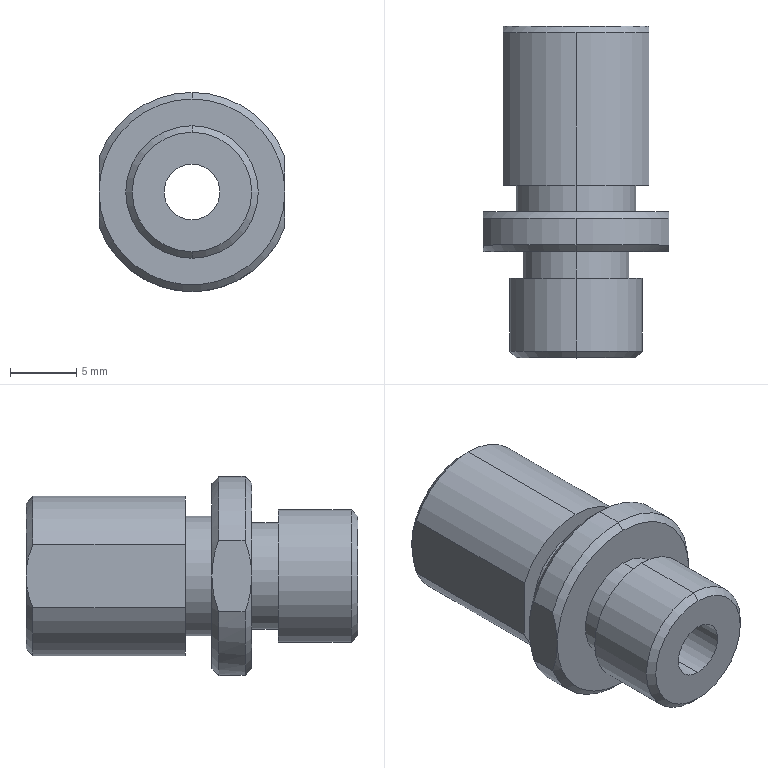Part | SolidWorks | features ICE 6, Chamfer 2, RevCut 2, Extrusion 1, MirrorPattern 1 | 1 solid | 35 faces | box 14 x 25 x 15 mm | volume 2174 mm3 | cylinder 14 | cone 11 | plane 10 | commonest cylinder face diameters 12 x3 15 x3 4.2 x2 8 x2 9 x2 10 x2
STEP:
#1=CARTESIAN_POINT('',(0.,-12.,-4.5));
#2=VERTEX_POINT('',#1);
#3=CARTESIAN_POINT('',(0.,-12.,4.5));
#4=VERTEX_POINT('',#3);
#5=CARTESIAN_POINT('',(0.,-12.,0.));
#6=DIRECTION('',(0.,-1.,0.));
#7=DIRECTION('',(0.,0.,-1.));
#8=AXIS2_PLACEMENT_3D('',#5,#6,#7);
#9=CIRCLE('',#8,4.5);
#10=EDGE_CURVE('',#2,#4,#9,.T.);
#11=ORIENTED_EDGE('',*,*,#10,.T.);
#12=CARTESIAN_POINT('',(0.,-14.,4.5));
#13=VERTEX_POINT('',#12);
#14=CARTESIAN_POINT('',(0.,-14.,4.5));
#15=DIRECTION('',(0.,-1.,0.));
#16=VECTOR('',#15,1000.);
#17=LINE('',#14,#16);
#18=EDGE_CURVE('',#4,#13,#17,.T.);
#19=ORIENTED_EDGE('',*,*,#18,.T.);
#20=CARTESIAN_POINT('',(0.,-14.,-4.5));
#21=VERTEX_POINT('',#20);
#22=CARTESIAN_POINT('',(0.,-14.,0.));
#23=DIRECTION('',(0.,-1.,0.));
#24=DIRECTION('',(0.,0.,-1.));
#25=AXIS2_PLACEMENT_3D('',#22,#23,#24);
#26=CIRCLE('',#25,4.5);
#27=EDGE_CURVE('',#21,#13,#26,.T.);
#28=ORIENTED_EDGE('',*,*,#27,.F.);
#29=CARTESIAN_POINT('',(0.,-14.,-4.5));
#30=DIRECTION('',(0.,-1.,0.));
#31=VECTOR('',#30,1000.);
#32=LINE('',#29,#31);
#33=EDGE_CURVE('',#2,#21,#32,.T.);
#34=ORIENTED_EDGE('',*,*,#33,.F.);
#35=EDGE_LOOP('',(#11,#19,#28,#34));
#36=FACE_OUTER_BOUND('',#35,.T.);
#37=CARTESIAN_POINT('',(0.,-14.,0.));
#38=DIRECTION('',(0.,-1.,0.));
#39=DIRECTION('',(0.,0.,-1.));
#40=AXIS2_PLACEMENT_3D('',#37,#38,#39);
#41=CYLINDRICAL_SURFACE('',#40,4.5);
#42=ADVANCED_FACE('',(#36),#41,.T.);
#43=CARTESIAN_POINT('',(0.,-17.,-4.));
#44=VERTEX_POINT('',#43);
#45=CARTESIAN_POINT('',(0.,-17.,4.));
#46=VERTEX_POINT('',#45);
#47=CARTESIAN_POINT('',(0.,-17.,0.));
#48=DIRECTION('',(0.,-1.,0.));
#49=DIRECTION('',(0.,0.,-1.));
#50=AXIS2_PLACEMENT_3D('',#47,#48,#49);
#51=CIRCLE('',#50,4.);
#52=EDGE_CURVE('',#44,#46,#51,.T.);
#53=ORIENTED_EDGE('',*,*,#52,.T.);
#54=CARTESIAN_POINT('',(0.,-19.,4.));
#55=VERTEX_POINT('',#54);
#56=CARTESIAN_POINT('',(0.,-16.5,4.));
#57=DIRECTION('',(0.,-1.,0.));
#58=VECTOR('',#57,1000.);
#59=LINE('',#56,#58);
#60=EDGE_CURVE('',#46,#55,#59,.T.);
#61=ORIENTED_EDGE('',*,*,#60,.T.);
#62=CARTESIAN_POINT('',(0.,-19.,-4.));
#63=VERTEX_POINT('',#62);
#64=CARTESIAN_POINT('',(0.,-19.,0.));
#65=DIRECTION('',(0.,-1.,0.));
#66=DIRECTION('',(0.,0.,-1.));
#67=AXIS2_PLACEMENT_3D('',#64,#65,#66);
#68=CIRCLE('',#67,4.);
#69=EDGE_CURVE('',#63,#55,#68,.T.);
#70=ORIENTED_EDGE('',*,*,#69,.F.);
#71=CARTESIAN_POINT('',(0.,-16.5,-4.));
#72=DIRECTION('',(0.,-1.,0.));
#73=VECTOR('',#72,1000.);
#74=LINE('',#71,#73);
#75=EDGE_CURVE('',#44,#63,#74,.T.);
#76=ORIENTED_EDGE('',*,*,#75,.F.);
#77=EDGE_LOOP('',(#53,#61,#70,#76));
#78=FACE_OUTER_BOUND('',#77,.T.);
#79=CARTESIAN_POINT('',(0.,-16.5,0.));
#80=DIRECTION('',(0.,-1.,0.));
#81=DIRECTION('',(0.,0.,-1.));
#82=AXIS2_PLACEMENT_3D('',#79,#80,#81);
#83=CYLINDRICAL_SURFACE('',#82,4.);
#84=ADVANCED_FACE('',(#78),#83,.T.);
#85=CARTESIAN_POINT('',(0.,-25.,-4.5));
#86=VERTEX_POINT('',#85);
#87=CARTESIAN_POINT('',(0.,-25.,4.5));
#88=VERTEX_POINT('',#87);
#89=CARTESIAN_POINT('',(0.,-25.,0.));
#90=DIRECTION('',(0.,-1.,0.));
#91=DIRECTION('',(0.,0.,-1.));
#92=AXIS2_PLACEMENT_3D('',#89,#90,#91);
#93=CIRCLE('',#92,4.5);
#94=EDGE_CURVE('',#86,#88,#93,.T.);
#95=ORIENTED_EDGE('',*,*,#94,.F.);
#96=CARTESIAN_POINT('',(0.,-24.5,-5.));
#97=VERTEX_POINT('',#96);
#98=CARTESIAN_POINT('',(0.,-25.,-4.5));
#99=DIRECTION('',(0.,0.7071,-0.7071));
#100=VECTOR('',#99,1000.);
#101=LINE('',#98,#100);
#102=EDGE_CURVE('',#86,#97,#101,.T.);
#103=ORIENTED_EDGE('',*,*,#102,.T.);
#104=CARTESIAN_POINT('',(0.,-24.5,5.));
#105=VERTEX_POINT('',#104);
#106=CARTESIAN_POINT('',(0.,-24.5,0.));
#107=DIRECTION('',(0.,1.,0.));
#108=DIRECTION('',(0.,0.,-1.));
#109=AXIS2_PLACEMENT_3D('',#106,#107,#108);
#110=CIRCLE('',#109,5.);
#111=EDGE_CURVE('',#105,#97,#110,.T.);
#112=ORIENTED_EDGE('',*,*,#111,.F.);
#113=CARTESIAN_POINT('',(0.,-25.,4.5));
#114=DIRECTION('',(0.,0.7071,0.7071));
#115=VECTOR('',#114,1000.);
#116=LINE('',#113,#115);
#117=EDGE_CURVE('',#88,#105,#116,.T.);
#118=ORIENTED_EDGE('',*,*,#117,.F.);
#119=EDGE_LOOP('',(#95,#103,#112,#118));
#120=FACE_OUTER_BOUND('',#119,.T.);
#121=CARTESIAN_POINT('',(0.,-25.,0.));
#122=DIRECTION('',(0.,1.,0.));
#123=DIRECTION('',(0.,0.,1.));
#124=AXIS2_PLACEMENT_3D('',#121,#122,#123);
#125=CONICAL_SURFACE('',#124,4.5,0.7854);
#126=ADVANCED_FACE('',(#120),#125,.T.);
#127=CARTESIAN_POINT('',(0.,0.,-5.5));
#128=VERTEX_POINT('',#127);
#129=CARTESIAN_POINT('',(-5.5,0.,0.));
#130=VERTEX_POINT('',#129);
#131=CARTESIAN_POINT('',(0.,0.,0.));
#132=DIRECTION('',(0.,1.,0.));
#133=DIRECTION('',(0.,0.,1.));
#134=AXIS2_PLACEMENT_3D('',#131,#132,#133);
#135=CIRCLE('',#134,5.5);
#136=EDGE_CURVE('',#128,#130,#135,.T.);
#137=ORIENTED_EDGE('',*,*,#136,.F.);
#138=CARTESIAN_POINT('',(0.,-0.5,-6.));
#139=VERTEX_POINT('',#138);
#140=CARTESIAN_POINT('',(0.,0.,-5.5));
#141=DIRECTION('',(0.,-0.7071,-0.7071));
#142=VECTOR('',#141,1000.);
#143=LINE('',#140,#142);
#144=EDGE_CURVE('',#128,#139,#143,.T.);
#145=ORIENTED_EDGE('',*,*,#144,.T.);
#146=CARTESIAN_POINT('',(-5.5,-0.5,-2.398));
#147=VERTEX_POINT('',#146);
#148=CARTESIAN_POINT('',(0.,-0.5,0.));
#149=DIRECTION('',(0.,-1.,0.));
#150=DIRECTION('',(0.,0.,1.));
#151=AXIS2_PLACEMENT_3D('',#148,#149,#150);
#152=CIRCLE('',#151,6.);
#153=EDGE_CURVE('',#147,#139,#152,.T.);
#154=ORIENTED_EDGE('',*,*,#153,.F.);
#155=CARTESIAN_POINT('',(-5.5,0.,0.));
#156=CARTESIAN_POINT('',(-5.5,0.,-0.4127));
#157=CARTESIAN_POINT('',(-5.5,-0.04687,-0.8197));
#158=CARTESIAN_POINT('',(-5.5,-0.1777,-1.423));
#159=CARTESIAN_POINT('',(-5.5,-0.2316,-1.623));
#160=CARTESIAN_POINT('',(-5.5,-0.3547,-2.016));
#161=CARTESIAN_POINT('',(-5.5,-0.4242,-2.208));
#162=CARTESIAN_POINT('',(-5.5,-0.5,-2.398));
#163=B_SPLINE_CURVE_WITH_KNOTS('',3,(#155,#156,#157,#158,#159,#160,#161,#162),.UNSPECIFIED.,.F.,.F.,(4,2,2,4),(0.006808,0.008026,0.008634,0.009243),.UNSPECIFIED.);
#164=EDGE_CURVE('',#130,#147,#163,.T.);
#165=ORIENTED_EDGE('',*,*,#164,.F.);
#166=EDGE_LOOP('',(#137,#145,#154,#165));
#167=FACE_OUTER_BOUND('',#166,.T.);
#168=CARTESIAN_POINT('',(0.,0.,0.));
#169=DIRECTION('',(0.,-1.,0.));
#170=DIRECTION('',(0.,0.,-1.));
#171=AXIS2_PLACEMENT_3D('',#168,#169,#170);
#172=CONICAL_SURFACE('',#171,5.5,0.7854);
#173=ADVANCED_FACE('',(#167),#172,.T.);
#174=CARTESIAN_POINT('',(0.,-25.,2.1));
#175=VERTEX_POINT('',#174);
#176=CARTESIAN_POINT('',(0.,-25.,-2.1));
#177=VERTEX_POINT('',#176);
#178=CARTESIAN_POINT('',(0.,-25.,0.));
#179=DIRECTION('',(0.,-1.,0.));
#180=DIRECTION('',(0.,0.,-1.));
#181=AXIS2_PLACEMENT_3D('',#178,#179,#180);
#182=CIRCLE('',#181,2.1);
#183=EDGE_CURVE('',#175,#177,#182,.T.);
#184=ORIENTED_EDGE('',*,*,#183,.T.);
#185=CARTESIAN_POINT('',(0.,0.,-2.1));
#186=VERTEX_POINT('',#185);
#187=CARTESIAN_POINT('',(0.,-25.,-2.1));
#188=DIRECTION('',(0.,1.,0.));
#189=VECTOR('',#188,1000.);
#190=LINE('',#187,#189);
#191=EDGE_CURVE('',#177,#186,#190,.T.);
#192=ORIENTED_EDGE('',*,*,#191,.T.);
#193=CARTESIAN_POINT('',(0.,0.,2.1));
#194=VERTEX_POINT('',#193);
#195=CARTESIAN_POINT('',(0.,0.,0.));
#196=DIRECTION('',(0.,-1.,0.));
#197=DIRECTION('',(0.,0.,-1.));
#198=AXIS2_PLACEMENT_3D('',#195,#196,#197);
#199=CIRCLE('',#198,2.1);
#200=EDGE_CURVE('',#194,#186,#199,.T.);
#201=ORIENTED_EDGE('',*,*,#200,.F.);
#202=CARTESIAN_POINT('',(0.,-25.,2.1));
#203=DIRECTION('',(0.,1.,0.));
#204=VECTOR('',#203,1000.);
#205=LINE('',#202,#204);
#206=EDGE_CURVE('',#175,#194,#205,.T.);
#207=ORIENTED_EDGE('',*,*,#206,.F.);
#208=EDGE_LOOP('',(#184,#192,#201,#207));
#209=FACE_OUTER_BOUND('',#208,.T.);
#210=CARTESIAN_POINT('',(0.,-25.,0.));
#211=DIRECTION('',(0.,1.,0.));
#212=DIRECTION('',(0.,0.,1.));
#213=AXIS2_PLACEMENT_3D('',#210,#211,#212);
#214=CYLINDRICAL_SURFACE('',#213,2.1);
#215=ADVANCED_FACE('',(#209),#214,.F.);
#216=CARTESIAN_POINT('',(0.,-14.,-7.));
#217=VERTEX_POINT('',#216);
#218=CARTESIAN_POINT('',(-7.,-14.,0.));
#219=VERTEX_POINT('',#218);
#220=CARTESIAN_POINT('',(0.,-14.,0.));
#221=DIRECTION('',(0.,1.,0.));
#222=DIRECTION('',(0.,0.,-1.));
#223=AXIS2_PLACEMENT_3D('',#220,#221,#222);
#224=CIRCLE('',#223,7.);
#225=EDGE_CURVE('',#217,#219,#224,.T.);
#226=ORIENTED_EDGE('',*,*,#225,.F.);
#227=CARTESIAN_POINT('',(0.,-14.5,-7.5));
#228=VERTEX_POINT('',#227);
#229=CARTESIAN_POINT('',(0.,-14.5,-7.5));
#230=DIRECTION('',(0.,-0.7071,-0.7071));
#231=VECTOR('',#230,1000.);
#232=LINE('',#229,#231);
#233=EDGE_CURVE('',#217,#228,#232,.T.);
#234=ORIENTED_EDGE('',*,*,#233,.T.);
#235=CARTESIAN_POINT('',(-7.,-14.5,-2.693));
#236=VERTEX_POINT('',#235);
#237=CARTESIAN_POINT('',(0.,-14.5,0.));
#238=DIRECTION('',(0.,-1.,0.));
#239=DIRECTION('',(0.,0.,-1.));
#240=AXIS2_PLACEMENT_3D('',#237,#238,#239);
#241=CIRCLE('',#240,7.5);
#242=EDGE_CURVE('',#236,#228,#241,.T.);
#243=ORIENTED_EDGE('',*,*,#242,.F.);
#244=CARTESIAN_POINT('',(-7.,-14.5,-2.693));
#245=CARTESIAN_POINT('',(-7.,-14.345,-2.26));
#246=CARTESIAN_POINT('',(-7.,-14.22,-1.821));
#247=CARTESIAN_POINT('',(-7.,-14.09,-1.148));
#248=CARTESIAN_POINT('',(-7.,-14.057,-0.9221));
#249=CARTESIAN_POINT('',(-7.,-14.012,-0.4642));
#250=CARTESIAN_POINT('',(-7.,-14.,-0.2312));
#251=CARTESIAN_POINT('',(-7.,-14.,0.));
#252=B_SPLINE_CURVE_WITH_KNOTS('',3,(#244,#245,#246,#247,#248,#249,#250,#251),.UNSPECIFIED.,.F.,.F.,(4,2,2,4),(0.008821,0.01018,0.01086,0.01154),.UNSPECIFIED.);
#253=EDGE_CURVE('',#236,#219,#252,.T.);
#254=ORIENTED_EDGE('',*,*,#253,.T.);
#255=EDGE_LOOP('',(#226,#234,#243,#254));
#256=FACE_OUTER_BOUND('',#255,.T.);
#257=CARTESIAN_POINT('',(0.,-14.5,0.));
#258=DIRECTION('',(0.,-1.,0.));
#259=DIRECTION('',(0.,0.,-1.));
#260=AXIS2_PLACEMENT_3D('',#257,#258,#259);
#261=CONICAL_SURFACE('',#260,7.5,0.7854);
#262=ADVANCED_FACE('',(#256),#261,.T.);
#263=CARTESIAN_POINT('',(0.,-17.,7.));
#264=VERTEX_POINT('',#263);
#265=CARTESIAN_POINT('',(-7.,-17.,0.));
#266=VERTEX_POINT('',#265);
#267=CARTESIAN_POINT('',(0.,-17.,0.));
#268=DIRECTION('',(0.,-1.,0.));
#269=DIRECTION('',(0.,0.,-1.));
#270=AXIS2_PLACEMENT_3D('',#267,#268,#269);
#271=CIRCLE('',#270,7.);
#272=EDGE_CURVE('',#264,#266,#271,.T.);
#273=ORIENTED_EDGE('',*,*,#272,.F.);
#274=CARTESIAN_POINT('',(0.,-16.5,7.5));
#275=VERTEX_POINT('',#274);
#276=CARTESIAN_POINT('',(0.,-17.,7.));
#277=DIRECTION('',(0.,0.7071,0.7071));
#278=VECTOR('',#277,1000.);
#279=LINE('',#276,#278);
#280=EDGE_CURVE('',#264,#275,#279,.T.);
#281=ORIENTED_EDGE('',*,*,#280,.T.);
#282=CARTESIAN_POINT('',(-7.,-16.5,2.693));
#283=VERTEX_POINT('',#282);
#284=CARTESIAN_POINT('',(0.,-16.5,0.));
#285=DIRECTION('',(0.,1.,0.));
#286=DIRECTION('',(0.,0.,-1.));
#287=AXIS2_PLACEMENT_3D('',#284,#285,#286);
#288=CIRCLE('',#287,7.5);
#289=EDGE_CURVE('',#283,#275,#288,.T.);
#290=ORIENTED_EDGE('',*,*,#289,.F.);
#291=CARTESIAN_POINT('',(-7.,-16.5,2.693));
#292=CARTESIAN_POINT('',(-7.,-16.656,2.257));
#293=CARTESIAN_POINT('',(-7.,-16.782,1.814));
#294=CARTESIAN_POINT('',(-7.,-16.954,0.9173));
#295=CARTESIAN_POINT('',(-7.,-17.,0.4625));
#296=CARTESIAN_POINT('',(-7.,-17.,0.));
#297=B_SPLINE_CURVE_WITH_KNOTS('',3,(#291,#292,#293,#294,#295,#296),.UNSPECIFIED.,.F.,.F.,(4,2,4),(0.005698,0.007064,0.008429),.UNSPECIFIED.);
#298=EDGE_CURVE('',#283,#266,#297,.T.);
#299=ORIENTED_EDGE('',*,*,#298,.T.);
#300=EDGE_LOOP('',(#273,#281,#290,#299));
#301=FACE_OUTER_BOUND('',#300,.T.);
#302=CARTESIAN_POINT('',(0.,-17.,0.));
#303=DIRECTION('',(0.,1.,0.));
#304=DIRECTION('',(0.,0.,1.));
#305=AXIS2_PLACEMENT_3D('',#302,#303,#304);
#306=CONICAL_SURFACE('',#305,7.,0.7854);
#307=ADVANCED_FACE('',(#301),#306,.T.);
#308=ORIENTED_EDGE('',*,*,#289,.T.);
#309=CARTESIAN_POINT('',(0.,-14.5,7.5));
#310=VERTEX_POINT('',#309);
#311=CARTESIAN_POINT('',(0.,-17.,7.5));
#312=DIRECTION('',(0.,1.,0.));
#313=VECTOR('',#312,1000.);
#314=LINE('',#311,#313);
#315=EDGE_CURVE('',#275,#310,#314,.T.);
#316=ORIENTED_EDGE('',*,*,#315,.T.);
#317=CARTESIAN_POINT('',(-7.,-14.5,2.693));
#318=VERTEX_POINT('',#317);
#319=CARTESIAN_POINT('',(0.,-14.5,0.));
#320=DIRECTION('',(0.,-1.,0.));
#321=DIRECTION('',(0.,0.,-1.));
#322=AXIS2_PLACEMENT_3D('',#319,#320,#321);
#323=CIRCLE('',#322,7.5);
#324=EDGE_CURVE('',#310,#318,#323,.T.);
#325=ORIENTED_EDGE('',*,*,#324,.T.);
#326=CARTESIAN_POINT('',(-7.,-17.,2.693));
#327=DIRECTION('',(0.,1.,0.));
#328=VECTOR('',#327,1000.);
#329=LINE('',#326,#328);
#330=EDGE_CURVE('',#283,#318,#329,.T.);
#331=ORIENTED_EDGE('',*,*,#330,.F.);
#332=EDGE_LOOP('',(#308,#316,#325,#331));
#333=FACE_OUTER_BOUND('',#332,.T.);
#334=CARTESIAN_POINT('',(0.,-17.,0.));
#335=DIRECTION('',(0.,1.,0.));
#336=DIRECTION('',(0.,0.,1.));
#337=AXIS2_PLACEMENT_3D('',#334,#335,#336);
#338=CYLINDRICAL_SURFACE('',#337,7.5);
#339=ADVANCED_FACE('',(#333),#338,.T.);
#340=ORIENTED_EDGE('',*,*,#111,.T.);
#341=CARTESIAN_POINT('',(0.,-19.,-5.));
#342=VERTEX_POINT('',#341);
#343=CARTESIAN_POINT('',(0.,-25.,-5.));
#344=DIRECTION('',(0.,1.,0.));
#345=VECTOR('',#344,1000.);
#346=LINE('',#343,#345);
#347=EDGE_CURVE('',#97,#342,#346,.T.);
#348=ORIENTED_EDGE('',*,*,#347,.T.);
#349=CARTESIAN_POINT('',(0.,-19.,5.));
#350=VERTEX_POINT('',#349);
#351=CARTESIAN_POINT('',(0.,-19.,0.));
#352=DIRECTION('',(0.,1.,0.));
#353=DIRECTION('',(0.,0.,1.));
#354=AXIS2_PLACEMENT_3D('',#351,#352,#353);
#355=CIRCLE('',#354,5.);
#356=EDGE_CURVE('',#350,#342,#355,.T.);
#357=ORIENTED_EDGE('',*,*,#356,.F.);
#358=CARTESIAN_POINT('',(0.,-25.,5.));
#359=DIRECTION('',(0.,1.,0.));
#360=VECTOR('',#359,1000.);
#361=LINE('',#358,#360);
#362=EDGE_CURVE('',#105,#350,#361,.T.);
#363=ORIENTED_EDGE('',*,*,#362,.F.);
#364=EDGE_LOOP('',(#340,#348,#357,#363));
#365=FACE_OUTER_BOUND('',#364,.T.);
#366=CARTESIAN_POINT('',(0.,-25.,0.));
#367=DIRECTION('',(0.,1.,0.));
#368=DIRECTION('',(0.,0.,1.));
#369=AXIS2_PLACEMENT_3D('',#366,#367,#368);
#370=CYLINDRICAL_SURFACE('',#369,5.);
#371=ADVANCED_FACE('',(#365),#370,.T.);
#372=CARTESIAN_POINT('',(-5.5,-12.,2.398));
#373=VERTEX_POINT('',#372);
#374=CARTESIAN_POINT('',(0.,-12.,6.));
#375=VERTEX_POINT('',#374);
#376=CARTESIAN_POINT('',(0.,-12.,0.));
#377=DIRECTION('',(0.,1.,0.));
#378=DIRECTION('',(0.,0.,-1.));
#379=AXIS2_PLACEMENT_3D('',#376,#377,#378);
#380=CIRCLE('',#379,6.);
#381=EDGE_CURVE('',#373,#375,#380,.T.);
#382=ORIENTED_EDGE('',*,*,#381,.T.);
#383=CARTESIAN_POINT('',(0.,-0.5,6.));
#384=VERTEX_POINT('',#383);
#385=CARTESIAN_POINT('',(0.,-14.,6.));
#386=DIRECTION('',(0.,1.,0.));
#387=VECTOR('',#386,1000.);
#388=LINE('',#385,#387);
#389=EDGE_CURVE('',#375,#384,#388,.T.);
#390=ORIENTED_EDGE('',*,*,#389,.T.);
#391=CARTESIAN_POINT('',(-5.5,-0.5,2.398));
#392=VERTEX_POINT('',#391);
#393=CARTESIAN_POINT('',(0.,-0.5,0.));
#394=DIRECTION('',(0.,-1.,0.));
#395=DIRECTION('',(0.,0.,1.));
#396=AXIS2_PLACEMENT_3D('',#393,#394,#395);
#397=CIRCLE('',#396,6.);
#398=EDGE_CURVE('',#384,#392,#397,.T.);
#399=ORIENTED_EDGE('',*,*,#398,.T.);
#400=CARTESIAN_POINT('',(-5.5,-14.,2.398));
#401=DIRECTION('',(0.,1.,0.));
#402=VECTOR('',#401,1000.);
#403=LINE('',#400,#402);
#404=EDGE_CURVE('',#373,#392,#403,.T.);
#405=ORIENTED_EDGE('',*,*,#404,.F.);
#406=EDGE_LOOP('',(#382,#390,#399,#405));
#407=FACE_OUTER_BOUND('',#406,.T.);
#408=CARTESIAN_POINT('',(0.,-14.,0.));
#409=DIRECTION('',(0.,1.,0.));
#410=DIRECTION('',(0.,0.,1.));
#411=AXIS2_PLACEMENT_3D('',#408,#409,#410);
#412=CYLINDRICAL_SURFACE('',#411,6.);
#413=ADVANCED_FACE('',(#407),#412,.T.);
#414=CARTESIAN_POINT('',(5.5,-12.,-2.398));
#415=VERTEX_POINT('',#414);
#416=CARTESIAN_POINT('',(5.5,-0.5,-2.398));
#417=VERTEX_POINT('',#416);
#418=CARTESIAN_POINT('',(5.5,-14.,-2.398));
#419=DIRECTION('',(0.,1.,0.));
#420=VECTOR('',#419,1000.);
#421=LINE('',#418,#420);
#422=EDGE_CURVE('',#415,#417,#421,.T.);
#423=ORIENTED_EDGE('',*,*,#422,.F.);
#424=CARTESIAN_POINT('',(-5.5,-12.,-2.398));
#425=VERTEX_POINT('',#424);
#426=CARTESIAN_POINT('',(0.,-12.,0.));
#427=DIRECTION('',(0.,1.,0.));
#428=DIRECTION('',(0.,0.,-1.));
#429=AXIS2_PLACEMENT_3D('',#426,#427,#428);
#430=CIRCLE('',#429,6.);
#431=EDGE_CURVE('',#415,#425,#430,.T.);
#432=ORIENTED_EDGE('',*,*,#431,.T.);
#433=CARTESIAN_POINT('',(-5.5,-14.,-2.398));
#434=DIRECTION('',(0.,-1.,0.));
#435=VECTOR('',#434,1000.);
#436=LINE('',#433,#435);
#437=EDGE_CURVE('',#147,#425,#436,.T.);
#438=ORIENTED_EDGE('',*,*,#437,.F.);
#439=ORIENTED_EDGE('',*,*,#153,.T.);
#440=CARTESIAN_POINT('',(0.,-0.5,0.));
#441=DIRECTION('',(0.,-1.,0.));
#442=DIRECTION('',(0.,0.,1.));
#443=AXIS2_PLACEMENT_3D('',#440,#441,#442);
#444=CIRCLE('',#443,6.);
#445=EDGE_CURVE('',#139,#417,#444,.T.);
#446=ORIENTED_EDGE('',*,*,#445,.T.);
#447=EDGE_LOOP('',(#423,#432,#438,#439,#446));
#448=FACE_OUTER_BOUND('',#447,.T.);
#449=CARTESIAN_POINT('',(0.,-14.,0.));
#450=DIRECTION('',(0.,1.,0.));
#451=DIRECTION('',(0.,0.,1.));
#452=AXIS2_PLACEMENT_3D('',#449,#450,#451);
#453=CYLINDRICAL_SURFACE('',#452,6.);
#454=ADVANCED_FACE('',(#448),#453,.T.);
#455=ORIENTED_EDGE('',*,*,#389,.F.);
#456=CARTESIAN_POINT('',(5.5,-12.,2.398));
#457=VERTEX_POINT('',#456);
#458=CARTESIAN_POINT('',(0.,-12.,0.));
#459=DIRECTION('',(0.,1.,0.));
#460=DIRECTION('',(0.,0.,-1.));
#461=AXIS2_PLACEMENT_3D('',#458,#459,#460);
#462=CIRCLE('',#461,6.);
#463=EDGE_CURVE('',#375,#457,#462,.T.);
#464=ORIENTED_EDGE('',*,*,#463,.T.);
#465=CARTESIAN_POINT('',(5.5,-0.5,2.398));
#466=VERTEX_POINT('',#465);
#467=CARTESIAN_POINT('',(5.5,-14.,2.398));
#468=DIRECTION('',(0.,-1.,0.));
#469=VECTOR('',#468,1000.);
#470=LINE('',#467,#469);
#471=EDGE_CURVE('',#466,#457,#470,.T.);
#472=ORIENTED_EDGE('',*,*,#471,.F.);
#473=CARTESIAN_POINT('',(0.,-0.5,0.));
#474=DIRECTION('',(0.,-1.,0.));
#475=DIRECTION('',(0.,0.,1.));
#476=AXIS2_PLACEMENT_3D('',#473,#474,#475);
#477=CIRCLE('',#476,6.);
#478=EDGE_CURVE('',#466,#384,#477,.T.);
#479=ORIENTED_EDGE('',*,*,#478,.T.);
#480=EDGE_LOOP('',(#455,#464,#472,#479));
#481=FACE_OUTER_BOUND('',#480,.T.);
#482=CARTESIAN_POINT('',(0.,-14.,0.));
#483=DIRECTION('',(0.,1.,0.));
#484=DIRECTION('',(0.,0.,1.));
#485=AXIS2_PLACEMENT_3D('',#482,#483,#484);
#486=CYLINDRICAL_SURFACE('',#485,6.);
#487=ADVANCED_FACE('',(#481),#486,.T.);
#488=CARTESIAN_POINT('',(5.5,-12.,-10.));
#489=DIRECTION('',(0.,0.,1.));
#490=VECTOR('',#489,1000.);
#491=LINE('',#488,#490);
#492=EDGE_CURVE('',#415,#457,#491,.T.);
#493=ORIENTED_EDGE('',*,*,#492,.F.);
#494=ORIENTED_EDGE('',*,*,#422,.T.);
#495=CARTESIAN_POINT('',(5.5,0.,0.));
#496=VERTEX_POINT('',#495);
#497=CARTESIAN_POINT('',(5.5,-0.5,-2.398));
#498=CARTESIAN_POINT('',(5.5,-0.4242,-2.208));
#499=CARTESIAN_POINT('',(5.5,-0.3547,-2.016));
#500=CARTESIAN_POINT('',(5.5,-0.2316,-1.623));
#501=CARTESIAN_POINT('',(5.5,-0.1777,-1.423));
#502=CARTESIAN_POINT('',(5.5,-0.04687,-0.8197));
#503=CARTESIAN_POINT('',(5.5,0.,-0.4127));
#504=CARTESIAN_POINT('',(5.5,0.,0.));
#505=B_SPLINE_CURVE_WITH_KNOTS('',3,(#497,#498,#499,#500,#501,#502,#503,#504),.UNSPECIFIED.,.F.,.F.,(4,2,2,4),(0.001956,0.002568,0.003181,0.004405),.UNSPECIFIED.);
#506=EDGE_CURVE('',#417,#496,#505,.T.);
#507=ORIENTED_EDGE('',*,*,#506,.T.);
#508=CARTESIAN_POINT('',(5.5,0.,0.));
#509=CARTESIAN_POINT('',(5.5,0.,0.2064));
#510=CARTESIAN_POINT('',(5.5,-0.0118,0.4135));
#511=CARTESIAN_POINT('',(5.5,-0.05728,0.8212));
#512=CARTESIAN_POINT('',(5.5,-0.0909,1.023));
#513=CARTESIAN_POINT('',(5.5,-0.2209,1.622));
#514=CARTESIAN_POINT('',(5.5,-0.3477,2.017));
#515=CARTESIAN_POINT('',(5.5,-0.5,2.398));
#516=B_SPLINE_CURVE_WITH_KNOTS('',3,(#508,#509,#510,#511,#512,#513,#514,#515),.UNSPECIFIED.,.F.,.F.,(4,2,2,4),(0.004405,0.005018,0.00563,0.006855),.UNSPECIFIED.);
#517=EDGE_CURVE('',#496,#466,#516,.T.);
#518=ORIENTED_EDGE('',*,*,#517,.T.);
#519=ORIENTED_EDGE('',*,*,#471,.T.);
#520=EDGE_LOOP('',(#493,#494,#507,#518,#519));
#521=FACE_OUTER_BOUND('',#520,.T.);
#522=CARTESIAN_POINT('',(5.5,13.542,-10.));
#523=DIRECTION('',(-1.,0.,0.));
#524=DIRECTION('',(0.,-1.,0.));
#525=AXIS2_PLACEMENT_3D('',#522,#523,#524);
#526=PLANE('',#525);
#527=ADVANCED_FACE('',(#521),#526,.F.);
#528=CARTESIAN_POINT('',(-5.5,-12.,-10.));
#529=DIRECTION('',(0.,0.,-1.));
#530=VECTOR('',#529,1000.);
#531=LINE('',#528,#530);
#532=EDGE_CURVE('',#373,#425,#531,.T.);
#533=ORIENTED_EDGE('',*,*,#532,.F.);
#534=ORIENTED_EDGE('',*,*,#404,.T.);
#535=CARTESIAN_POINT('',(-5.5,-0.5,2.398));
#536=CARTESIAN_POINT('',(-5.5,-0.3477,2.017));
#537=CARTESIAN_POINT('',(-5.5,-0.2209,1.622));
#538=CARTESIAN_POINT('',(-5.5,-0.0909,1.023));
#539=CARTESIAN_POINT('',(-5.5,-0.05728,0.8212));
#540=CARTESIAN_POINT('',(-5.5,-0.0118,0.4135));
#541=CARTESIAN_POINT('',(-5.5,0.,0.2064));
#542=CARTESIAN_POINT('',(-5.5,0.,0.));
#543=B_SPLINE_CURVE_WITH_KNOTS('',3,(#535,#536,#537,#538,#539,#540,#541,#542),.UNSPECIFIED.,.F.,.F.,(4,2,2,4),(0.004372,0.00559,0.006199,0.006808),.UNSPECIFIED.);
#544=EDGE_CURVE('',#392,#130,#543,.T.);
#545=ORIENTED_EDGE('',*,*,#544,.T.);
#546=ORIENTED_EDGE('',*,*,#164,.T.);
#547=ORIENTED_EDGE('',*,*,#437,.T.);
#548=EDGE_LOOP('',(#533,#534,#545,#546,#547));
#549=FACE_OUTER_BOUND('',#548,.T.);
#550=CARTESIAN_POINT('',(-5.5,13.542,-10.));
#551=DIRECTION('',(1.,0.,0.));
#552=DIRECTION('',(0.,1.,0.));
#553=AXIS2_PLACEMENT_3D('',#550,#551,#552);
#554=PLANE('',#553);
#555=ADVANCED_FACE('',(#549),#554,.F.);
#556=ORIENTED_EDGE('',*,*,#347,.F.);
#557=CARTESIAN_POINT('',(0.,-24.5,0.));
#558=DIRECTION('',(0.,1.,0.));
#559=DIRECTION('',(0.,0.,-1.));
#560=AXIS2_PLACEMENT_3D('',#557,#558,#559);
#561=CIRCLE('',#560,5.);
#562=EDGE_CURVE('',#97,#105,#561,.T.);
#563=ORIENTED_EDGE('',*,*,#562,.T.);
#564=ORIENTED_EDGE('',*,*,#362,.T.);
#565=CARTESIAN_POINT('',(0.,-19.,0.));
#566=DIRECTION('',(0.,1.,0.));
#567=DIRECTION('',(0.,0.,1.));
#568=AXIS2_PLACEMENT_3D('',#565,#566,#567);
#569=CIRCLE('',#568,5.);
#570=EDGE_CURVE('',#342,#350,#569,.T.);
#571=ORIENTED_EDGE('',*,*,#570,.F.);
#572=EDGE_LOOP('',(#556,#563,#564,#571));
#573=FACE_OUTER_BOUND('',#572,.T.);
#574=CARTESIAN_POINT('',(0.,-25.,0.));
#575=DIRECTION('',(0.,1.,0.));
#576=DIRECTION('',(0.,0.,1.));
#577=AXIS2_PLACEMENT_3D('',#574,#575,#576);
#578=CYLINDRICAL_SURFACE('',#577,5.);
#579=ADVANCED_FACE('',(#573),#578,.T.);
#580=ORIENTED_EDGE('',*,*,#544,.F.);
#581=ORIENTED_EDGE('',*,*,#398,.F.);
#582=ORIENTED_EDGE('',*,*,#478,.F.);
#583=ORIENTED_EDGE('',*,*,#517,.F.);
#584=CARTESIAN_POINT('',(0.,0.,0.));
#585=DIRECTION('',(0.,1.,0.));
#586=DIRECTION('',(0.,0.,1.));
#587=AXIS2_PLACEMENT_3D('',#584,#585,#586);
#588=CIRCLE('',#587,5.5);
#589=EDGE_CURVE('',#130,#496,#588,.T.);
#590=ORIENTED_EDGE('',*,*,#589,.F.);
#591=EDGE_LOOP('',(#580,#581,#582,#583,#590));
#592=FACE_OUTER_BOUND('',#591,.T.);
#593=CARTESIAN_POINT('',(0.,0.,0.));
#594=DIRECTION('',(0.,-1.,0.));
#595=DIRECTION('',(0.,0.,-1.));
#596=AXIS2_PLACEMENT_3D('',#593,#594,#595);
#597=CONICAL_SURFACE('',#596,5.5,0.7854);
#598=ADVANCED_FACE('',(#592),#597,.T.);
#599=ORIENTED_EDGE('',*,*,#315,.F.);
#600=CARTESIAN_POINT('',(7.,-16.5,2.693));
#601=VERTEX_POINT('',#600);
#602=CARTESIAN_POINT('',(0.,-16.5,0.));
#603=DIRECTION('',(0.,1.,0.));
#604=DIRECTION('',(0.,0.,-1.));
#605=AXIS2_PLACEMENT_3D('',#602,#603,#604);
#606=CIRCLE('',#605,7.5);
#607=EDGE_CURVE('',#275,#601,#606,.T.);
#608=ORIENTED_EDGE('',*,*,#607,.T.);
#609=CARTESIAN_POINT('',(7.,-14.5,2.693));
#610=VERTEX_POINT('',#609);
#611=CARTESIAN_POINT('',(7.,-17.,2.693));
#612=DIRECTION('',(0.,1.,0.));
#613=VECTOR('',#612,1000.);
#614=LINE('',#611,#613);
#615=EDGE_CURVE('',#601,#610,#614,.T.);
#616=ORIENTED_EDGE('',*,*,#615,.T.);
#617=CARTESIAN_POINT('',(0.,-14.5,0.));
#618=DIRECTION('',(0.,-1.,0.));
#619=DIRECTION('',(0.,0.,-1.));
#620=AXIS2_PLACEMENT_3D('',#617,#618,#619);
#621=CIRCLE('',#620,7.5);
#622=EDGE_CURVE('',#610,#310,#621,.T.);
#623=ORIENTED_EDGE('',*,*,#622,.T.);
#624=EDGE_LOOP('',(#599,#608,#616,#623));
#625=FACE_OUTER_BOUND('',#624,.T.);
#626=CARTESIAN_POINT('',(0.,-17.,0.));
#627=DIRECTION('',(0.,1.,0.));
#628=DIRECTION('',(0.,0.,1.));
#629=AXIS2_PLACEMENT_3D('',#626,#627,#628);
#630=CYLINDRICAL_SURFACE('',#629,7.5);
#631=ADVANCED_FACE('',(#625),#630,.T.);
#632=CARTESIAN_POINT('',(-7.,-16.5,-2.693));
#633=VERTEX_POINT('',#632);
#634=CARTESIAN_POINT('',(-7.,-17.,-2.693));
#635=DIRECTION('',(0.,-1.,0.));
#636=VECTOR('',#635,1000.);
#637=LINE('',#634,#636);
#638=EDGE_CURVE('',#236,#633,#637,.T.);
#639=ORIENTED_EDGE('',*,*,#638,.F.);
#640=ORIENTED_EDGE('',*,*,#242,.T.);
#641=CARTESIAN_POINT('',(7.,-14.5,-2.693));
#642=VERTEX_POINT('',#641);
#643=CARTESIAN_POINT('',(0.,-14.5,0.));
#644=DIRECTION('',(0.,-1.,0.));
#645=DIRECTION('',(0.,0.,-1.));
#646=AXIS2_PLACEMENT_3D('',#643,#644,#645);
#647=CIRCLE('',#646,7.5);
#648=EDGE_CURVE('',#228,#642,#647,.T.);
#649=ORIENTED_EDGE('',*,*,#648,.T.);
#650=CARTESIAN_POINT('',(7.,-16.5,-2.693));
#651=VERTEX_POINT('',#650);
#652=CARTESIAN_POINT('',(7.,-17.,-2.693));
#653=DIRECTION('',(0.,-1.,0.));
#654=VECTOR('',#653,1000.);
#655=LINE('',#652,#654);
#656=EDGE_CURVE('',#642,#651,#655,.T.);
#657=ORIENTED_EDGE('',*,*,#656,.T.);
#658=CARTESIAN_POINT('',(0.,-16.5,0.));
#659=DIRECTION('',(0.,1.,0.));
#660=DIRECTION('',(0.,0.,-1.));
#661=AXIS2_PLACEMENT_3D('',#658,#659,#660);
#662=CIRCLE('',#661,7.5);
#663=EDGE_CURVE('',#651,#633,#662,.T.);
#664=ORIENTED_EDGE('',*,*,#663,.T.);
#665=EDGE_LOOP('',(#639,#640,#649,#657,#664));
#666=FACE_OUTER_BOUND('',#665,.T.);
#667=CARTESIAN_POINT('',(0.,-17.,0.));
#668=DIRECTION('',(0.,1.,0.));
#669=DIRECTION('',(0.,0.,1.));
#670=AXIS2_PLACEMENT_3D('',#667,#668,#669);
#671=CYLINDRICAL_SURFACE('',#670,7.5);
#672=ADVANCED_FACE('',(#666),#671,.T.);
#673=ORIENTED_EDGE('',*,*,#280,.F.);
#674=CARTESIAN_POINT('',(7.,-17.,0.));
#675=VERTEX_POINT('',#674);
#676=CARTESIAN_POINT('',(0.,-17.,0.));
#677=DIRECTION('',(0.,-1.,0.));
#678=DIRECTION('',(0.,0.,-1.));
#679=AXIS2_PLACEMENT_3D('',#676,#677,#678);
#680=CIRCLE('',#679,7.);
#681=EDGE_CURVE('',#675,#264,#680,.T.);
#682=ORIENTED_EDGE('',*,*,#681,.F.);
#683=CARTESIAN_POINT('',(7.,-16.5,2.693));
#684=CARTESIAN_POINT('',(7.,-16.656,2.257));
#685=CARTESIAN_POINT('',(7.,-16.782,1.814));
#686=CARTESIAN_POINT('',(7.,-16.954,0.9173));
#687=CARTESIAN_POINT('',(7.,-17.,0.4625));
#688=CARTESIAN_POINT('',(7.,-17.,0.));
#689=B_SPLINE_CURVE_WITH_KNOTS('',3,(#683,#684,#685,#686,#687,#688),.UNSPECIFIED.,.F.,.F.,(4,2,4),(0.005698,0.007064,0.008429),.UNSPECIFIED.);
#690=EDGE_CURVE('',#601,#675,#689,.T.);
#691=ORIENTED_EDGE('',*,*,#690,.F.);
#692=ORIENTED_EDGE('',*,*,#607,.F.);
#693=EDGE_LOOP('',(#673,#682,#691,#692));
#694=FACE_OUTER_BOUND('',#693,.T.);
#695=CARTESIAN_POINT('',(0.,-17.,0.));
#696=DIRECTION('',(0.,1.,0.));
#697=DIRECTION('',(0.,0.,1.));
#698=AXIS2_PLACEMENT_3D('',#695,#696,#697);
#699=CONICAL_SURFACE('',#698,7.,0.7854);
#700=ADVANCED_FACE('',(#694),#699,.T.);
#701=CARTESIAN_POINT('',(0.,-17.,0.));
#702=DIRECTION('',(0.,-1.,0.));
#703=DIRECTION('',(0.,0.,-1.));
#704=AXIS2_PLACEMENT_3D('',#701,#702,#703);
#705=CIRCLE('',#704,7.);
#706=EDGE_CURVE('',#266,#675,#705,.T.);
#707=ORIENTED_EDGE('',*,*,#706,.F.);
#708=CARTESIAN_POINT('',(-7.,-17.,0.));
#709=CARTESIAN_POINT('',(-7.,-17.,-0.2312));
#710=CARTESIAN_POINT('',(-7.,-16.988,-0.4642));
#711=CARTESIAN_POINT('',(-7.,-16.943,-0.9221));
#712=CARTESIAN_POINT('',(-7.,-16.91,-1.148));
#713=CARTESIAN_POINT('',(-7.,-16.78,-1.821));
#714=CARTESIAN_POINT('',(-7.,-16.655,-2.26));
#715=CARTESIAN_POINT('',(-7.,-16.5,-2.693));
#716=B_SPLINE_CURVE_WITH_KNOTS('',3,(#708,#709,#710,#711,#712,#713,#714,#715),.UNSPECIFIED.,.F.,.F.,(4,2,2,4),(0.008429,0.009112,0.009795,0.01116),.UNSPECIFIED.);
#717=EDGE_CURVE('',#266,#633,#716,.T.);
#718=ORIENTED_EDGE('',*,*,#717,.T.);
#719=ORIENTED_EDGE('',*,*,#663,.F.);
#720=CARTESIAN_POINT('',(7.,-17.,0.));
#721=CARTESIAN_POINT('',(7.,-17.,-0.2312));
#722=CARTESIAN_POINT('',(7.,-16.988,-0.4642));
#723=CARTESIAN_POINT('',(7.,-16.943,-0.9221));
#724=CARTESIAN_POINT('',(7.,-16.91,-1.148));
#725=CARTESIAN_POINT('',(7.,-16.78,-1.821));
#726=CARTESIAN_POINT('',(7.,-16.655,-2.26));
#727=CARTESIAN_POINT('',(7.,-16.5,-2.693));
#728=B_SPLINE_CURVE_WITH_KNOTS('',3,(#720,#721,#722,#723,#724,#725,#726,#727),.UNSPECIFIED.,.F.,.F.,(4,2,2,4),(0.008429,0.009112,0.009795,0.01116),.UNSPECIFIED.);
#729=EDGE_CURVE('',#675,#651,#728,.T.);
#730=ORIENTED_EDGE('',*,*,#729,.F.);
#731=EDGE_LOOP('',(#707,#718,#719,#730));
#732=FACE_OUTER_BOUND('',#731,.T.);
#733=CARTESIAN_POINT('',(0.,-17.,0.));
#734=DIRECTION('',(0.,1.,0.));
#735=DIRECTION('',(0.,0.,1.));
#736=AXIS2_PLACEMENT_3D('',#733,#734,#735);
#737=CONICAL_SURFACE('',#736,7.,0.7854);
#738=ADVANCED_FACE('',(#732),#737,.T.);
#739=ORIENTED_EDGE('',*,*,#233,.F.);
#740=CARTESIAN_POINT('',(7.,-14.,0.));
#741=VERTEX_POINT('',#740);
#742=CARTESIAN_POINT('',(0.,-14.,0.));
#743=DIRECTION('',(0.,1.,0.));
#744=DIRECTION('',(0.,0.,-1.));
#745=AXIS2_PLACEMENT_3D('',#742,#743,#744);
#746=CIRCLE('',#745,7.);
#747=EDGE_CURVE('',#741,#217,#746,.T.);
#748=ORIENTED_EDGE('',*,*,#747,.F.);
#749=CARTESIAN_POINT('',(7.,-14.5,-2.693));
#750=CARTESIAN_POINT('',(7.,-14.345,-2.26));
#751=CARTESIAN_POINT('',(7.,-14.22,-1.821));
#752=CARTESIAN_POINT('',(7.,-14.09,-1.148));
#753=CARTESIAN_POINT('',(7.,-14.057,-0.9221));
#754=CARTESIAN_POINT('',(7.,-14.012,-0.4642));
#755=CARTESIAN_POINT('',(7.,-14.,-0.2312));
#756=CARTESIAN_POINT('',(7.,-14.,0.));
#757=B_SPLINE_CURVE_WITH_KNOTS('',3,(#749,#750,#751,#752,#753,#754,#755,#756),.UNSPECIFIED.,.F.,.F.,(4,2,2,4),(0.008821,0.01018,0.01086,0.01154),.UNSPECIFIED.);
#758=EDGE_CURVE('',#642,#741,#757,.T.);
#759=ORIENTED_EDGE('',*,*,#758,.F.);
#760=ORIENTED_EDGE('',*,*,#648,.F.);
#761=EDGE_LOOP('',(#739,#748,#759,#760));
#762=FACE_OUTER_BOUND('',#761,.T.);
#763=CARTESIAN_POINT('',(0.,-14.5,0.));
#764=DIRECTION('',(0.,-1.,0.));
#765=DIRECTION('',(0.,0.,-1.));
#766=AXIS2_PLACEMENT_3D('',#763,#764,#765);
#767=CONICAL_SURFACE('',#766,7.5,0.7854);
#768=ADVANCED_FACE('',(#762),#767,.T.);
#769=CARTESIAN_POINT('',(0.,-14.,0.));
#770=DIRECTION('',(0.,1.,0.));
#771=DIRECTION('',(0.,0.,-1.));
#772=AXIS2_PLACEMENT_3D('',#769,#770,#771);
#773=CIRCLE('',#772,7.);
#774=EDGE_CURVE('',#219,#741,#773,.T.);
#775=ORIENTED_EDGE('',*,*,#774,.F.);
#776=CARTESIAN_POINT('',(-7.,-14.,0.));
#777=CARTESIAN_POINT('',(-7.,-14.,0.4625));
#778=CARTESIAN_POINT('',(-7.,-14.046,0.9173));
#779=CARTESIAN_POINT('',(-7.,-14.218,1.814));
#780=CARTESIAN_POINT('',(-7.,-14.344,2.257));
#781=CARTESIAN_POINT('',(-7.,-14.5,2.693));
#782=B_SPLINE_CURVE_WITH_KNOTS('',3,(#776,#777,#778,#779,#780,#781),.UNSPECIFIED.,.F.,.F.,(4,2,4),(0.01154,0.0129,0.01427),.UNSPECIFIED.);
#783=EDGE_CURVE('',#219,#318,#782,.T.);
#784=ORIENTED_EDGE('',*,*,#783,.T.);
#785=ORIENTED_EDGE('',*,*,#324,.F.);
#786=ORIENTED_EDGE('',*,*,#622,.F.);
#787=CARTESIAN_POINT('',(7.,-14.,0.));
#788=CARTESIAN_POINT('',(7.,-14.,0.4625));
#789=CARTESIAN_POINT('',(7.,-14.046,0.9173));
#790=CARTESIAN_POINT('',(7.,-14.218,1.814));
#791=CARTESIAN_POINT('',(7.,-14.344,2.257));
#792=CARTESIAN_POINT('',(7.,-14.5,2.693));
#793=B_SPLINE_CURVE_WITH_KNOTS('',3,(#787,#788,#789,#790,#791,#792),.UNSPECIFIED.,.F.,.F.,(4,2,4),(0.01154,0.0129,0.01427),.UNSPECIFIED.);
#794=EDGE_CURVE('',#741,#610,#793,.T.);
#795=ORIENTED_EDGE('',*,*,#794,.F.);
#796=EDGE_LOOP('',(#775,#784,#785,#786,#795));
#797=FACE_OUTER_BOUND('',#796,.T.);
#798=CARTESIAN_POINT('',(0.,-14.5,0.));
#799=DIRECTION('',(0.,-1.,0.));
#800=DIRECTION('',(0.,0.,-1.));
#801=AXIS2_PLACEMENT_3D('',#798,#799,#800);
#802=CONICAL_SURFACE('',#801,7.5,0.7854);
#803=ADVANCED_FACE('',(#797),#802,.T.);
#804=CARTESIAN_POINT('',(0.,0.,0.));
#805=DIRECTION('',(0.,1.,0.));
#806=DIRECTION('',(0.,0.,1.));
#807=AXIS2_PLACEMENT_3D('',#804,#805,#806);
#808=CIRCLE('',#807,5.5);
#809=EDGE_CURVE('',#496,#128,#808,.T.);
#810=ORIENTED_EDGE('',*,*,#809,.T.);
#811=ORIENTED_EDGE('',*,*,#136,.T.);
#812=ORIENTED_EDGE('',*,*,#589,.T.);
#813=EDGE_LOOP('',(#810,#811,#812));
#814=FACE_OUTER_BOUND('',#813,.T.);
#815=ORIENTED_EDGE('',*,*,#200,.T.);
#816=CARTESIAN_POINT('',(0.,0.,0.));
#817=DIRECTION('',(0.,-1.,0.));
#818=DIRECTION('',(0.,0.,-1.));
#819=AXIS2_PLACEMENT_3D('',#816,#817,#818);
#820=CIRCLE('',#819,2.1);
#821=EDGE_CURVE('',#186,#194,#820,.T.);
#822=ORIENTED_EDGE('',*,*,#821,.T.);
#823=EDGE_LOOP('',(#815,#822));
#824=FACE_BOUND('',#823,.T.);
#825=CARTESIAN_POINT('',(0.,0.,0.));
#826=DIRECTION('',(0.,1.,0.));
#827=DIRECTION('',(0.,0.,1.));
#828=AXIS2_PLACEMENT_3D('',#825,#826,#827);
#829=PLANE('',#828);
#830=ADVANCED_FACE('',(#814,#824),#829,.T.);
#831=CARTESIAN_POINT('',(0.,-25.,0.));
#832=DIRECTION('',(0.,-1.,0.));
#833=DIRECTION('',(0.,0.,-1.));
#834=AXIS2_PLACEMENT_3D('',#831,#832,#833);
#835=CIRCLE('',#834,4.5);
#836=EDGE_CURVE('',#88,#86,#835,.T.);
#837=ORIENTED_EDGE('',*,*,#836,.T.);
#838=ORIENTED_EDGE('',*,*,#94,.T.);
#839=EDGE_LOOP('',(#837,#838));
#840=FACE_OUTER_BOUND('',#839,.T.);
#841=ORIENTED_EDGE('',*,*,#183,.F.);
#842=CARTESIAN_POINT('',(0.,-25.,0.));
#843=DIRECTION('',(0.,-1.,0.));
#844=DIRECTION('',(0.,0.,-1.));
#845=AXIS2_PLACEMENT_3D('',#842,#843,#844);
#846=CIRCLE('',#845,2.1);
#847=EDGE_CURVE('',#177,#175,#846,.T.);
#848=ORIENTED_EDGE('',*,*,#847,.F.);
#849=EDGE_LOOP('',(#841,#848));
#850=FACE_BOUND('',#849,.T.);
#851=CARTESIAN_POINT('',(0.,-25.,0.));
#852=DIRECTION('',(0.,-1.,0.));
#853=DIRECTION('',(0.,0.,-1.));
#854=AXIS2_PLACEMENT_3D('',#851,#852,#853);
#855=PLANE('',#854);
#856=ADVANCED_FACE('',(#840,#850),#855,.T.);
#857=ORIENTED_EDGE('',*,*,#681,.T.);
#858=ORIENTED_EDGE('',*,*,#272,.T.);
#859=ORIENTED_EDGE('',*,*,#706,.T.);
#860=EDGE_LOOP('',(#857,#858,#859));
#861=FACE_OUTER_BOUND('',#860,.T.);
#862=ORIENTED_EDGE('',*,*,#52,.F.);
#863=CARTESIAN_POINT('',(0.,-17.,0.));
#864=DIRECTION('',(0.,-1.,0.));
#865=DIRECTION('',(0.,0.,-1.));
#866=AXIS2_PLACEMENT_3D('',#863,#864,#865);
#867=CIRCLE('',#866,4.);
#868=EDGE_CURVE('',#46,#44,#867,.T.);
#869=ORIENTED_EDGE('',*,*,#868,.F.);
#870=EDGE_LOOP('',(#862,#869));
#871=FACE_BOUND('',#870,.T.);
#872=CARTESIAN_POINT('',(0.,-17.,0.));
#873=DIRECTION('',(0.,-1.,0.));
#874=DIRECTION('',(0.,0.,-1.));
#875=AXIS2_PLACEMENT_3D('',#872,#873,#874);
#876=PLANE('',#875);
#877=ADVANCED_FACE('',(#861,#871),#876,.T.);
#878=ORIENTED_EDGE('',*,*,#747,.T.);
#879=ORIENTED_EDGE('',*,*,#225,.T.);
#880=ORIENTED_EDGE('',*,*,#774,.T.);
#881=EDGE_LOOP('',(#878,#879,#880));
#882=FACE_OUTER_BOUND('',#881,.T.);
#883=ORIENTED_EDGE('',*,*,#27,.T.);
#884=CARTESIAN_POINT('',(0.,-14.,0.));
#885=DIRECTION('',(0.,-1.,0.));
#886=DIRECTION('',(0.,0.,-1.));
#887=AXIS2_PLACEMENT_3D('',#884,#885,#886);
#888=CIRCLE('',#887,4.5);
#889=EDGE_CURVE('',#13,#21,#888,.T.);
#890=ORIENTED_EDGE('',*,*,#889,.T.);
#891=EDGE_LOOP('',(#883,#890));
#892=FACE_BOUND('',#891,.T.);
#893=CARTESIAN_POINT('',(0.,-14.,0.));
#894=DIRECTION('',(0.,-1.,0.));
#895=DIRECTION('',(0.,0.,-1.));
#896=AXIS2_PLACEMENT_3D('',#893,#894,#895);
#897=PLANE('',#896);
#898=ADVANCED_FACE('',(#882,#892),#897,.F.);
#899=ORIENTED_EDGE('',*,*,#191,.F.);
#900=ORIENTED_EDGE('',*,*,#847,.T.);
#901=ORIENTED_EDGE('',*,*,#206,.T.);
#902=ORIENTED_EDGE('',*,*,#821,.F.);
#903=EDGE_LOOP('',(#899,#900,#901,#902));
#904=FACE_OUTER_BOUND('',#903,.T.);
#905=CARTESIAN_POINT('',(0.,-25.,0.));
#906=DIRECTION('',(0.,1.,0.));
#907=DIRECTION('',(0.,0.,1.));
#908=AXIS2_PLACEMENT_3D('',#905,#906,#907);
#909=CYLINDRICAL_SURFACE('',#908,2.1);
#910=ADVANCED_FACE('',(#904),#909,.F.);
#911=ORIENTED_EDGE('',*,*,#144,.F.);
#912=ORIENTED_EDGE('',*,*,#809,.F.);
#913=ORIENTED_EDGE('',*,*,#506,.F.);
#914=ORIENTED_EDGE('',*,*,#445,.F.);
#915=EDGE_LOOP('',(#911,#912,#913,#914));
#916=FACE_OUTER_BOUND('',#915,.T.);
#917=CARTESIAN_POINT('',(0.,0.,0.));
#918=DIRECTION('',(0.,-1.,0.));
#919=DIRECTION('',(0.,0.,-1.));
#920=AXIS2_PLACEMENT_3D('',#917,#918,#919);
#921=CONICAL_SURFACE('',#920,5.5,0.7854);
#922=ADVANCED_FACE('',(#916),#921,.T.);
#923=ORIENTED_EDGE('',*,*,#690,.T.);
#924=ORIENTED_EDGE('',*,*,#729,.T.);
#925=ORIENTED_EDGE('',*,*,#656,.F.);
#926=ORIENTED_EDGE('',*,*,#758,.T.);
#927=ORIENTED_EDGE('',*,*,#794,.T.);
#928=ORIENTED_EDGE('',*,*,#615,.F.);
#929=EDGE_LOOP('',(#923,#924,#925,#926,#927,#928));
#930=FACE_OUTER_BOUND('',#929,.T.);
#931=CARTESIAN_POINT('',(7.,-4.135,-4.5));
#932=DIRECTION('',(-1.,0.,0.));
#933=DIRECTION('',(0.,-1.,0.));
#934=AXIS2_PLACEMENT_3D('',#931,#932,#933);
#935=PLANE('',#934);
#936=ADVANCED_FACE('',(#930),#935,.F.);
#937=ORIENTED_EDGE('',*,*,#330,.T.);
#938=ORIENTED_EDGE('',*,*,#783,.F.);
#939=ORIENTED_EDGE('',*,*,#253,.F.);
#940=ORIENTED_EDGE('',*,*,#638,.T.);
#941=ORIENTED_EDGE('',*,*,#717,.F.);
#942=ORIENTED_EDGE('',*,*,#298,.F.);
#943=EDGE_LOOP('',(#937,#938,#939,#940,#941,#942));
#944=FACE_OUTER_BOUND('',#943,.T.);
#945=CARTESIAN_POINT('',(-7.,-4.135,-4.5));
#946=DIRECTION('',(-1.,0.,0.));
#947=DIRECTION('',(0.,-1.,0.));
#948=AXIS2_PLACEMENT_3D('',#945,#946,#947);
#949=PLANE('',#948);
#950=ADVANCED_FACE('',(#944),#949,.T.);
#951=ORIENTED_EDGE('',*,*,#102,.F.);
#952=ORIENTED_EDGE('',*,*,#836,.F.);
#953=ORIENTED_EDGE('',*,*,#117,.T.);
#954=ORIENTED_EDGE('',*,*,#562,.F.);
#955=EDGE_LOOP('',(#951,#952,#953,#954));
#956=FACE_OUTER_BOUND('',#955,.T.);
#957=CARTESIAN_POINT('',(0.,-25.,0.));
#958=DIRECTION('',(0.,1.,0.));
#959=DIRECTION('',(0.,0.,1.));
#960=AXIS2_PLACEMENT_3D('',#957,#958,#959);
#961=CONICAL_SURFACE('',#960,4.5,0.7854);
#962=ADVANCED_FACE('',(#956),#961,.T.);
#963=ORIENTED_EDGE('',*,*,#69,.T.);
#964=CARTESIAN_POINT('',(0.,-19.,0.));
#965=DIRECTION('',(0.,-1.,0.));
#966=DIRECTION('',(0.,0.,-1.));
#967=AXIS2_PLACEMENT_3D('',#964,#965,#966);
#968=CIRCLE('',#967,4.);
#969=EDGE_CURVE('',#55,#63,#968,.T.);
#970=ORIENTED_EDGE('',*,*,#969,.T.);
#971=EDGE_LOOP('',(#963,#970));
#972=FACE_BOUND('',#971,.T.);
#973=ORIENTED_EDGE('',*,*,#356,.T.);
#974=ORIENTED_EDGE('',*,*,#570,.T.);
#975=EDGE_LOOP('',(#973,#974));
#976=FACE_OUTER_BOUND('',#975,.T.);
#977=CARTESIAN_POINT('',(-13.293,-19.,0.));
#978=DIRECTION('',(0.,1.,0.));
#979=DIRECTION('',(0.,0.,1.));
#980=AXIS2_PLACEMENT_3D('',#977,#978,#979);
#981=PLANE('',#980);
#982=ADVANCED_FACE('',(#972,#976),#981,.T.);
#983=ORIENTED_EDGE('',*,*,#60,.F.);
#984=ORIENTED_EDGE('',*,*,#868,.T.);
#985=ORIENTED_EDGE('',*,*,#75,.T.);
#986=ORIENTED_EDGE('',*,*,#969,.F.);
#987=EDGE_LOOP('',(#983,#984,#985,#986));
#988=FACE_OUTER_BOUND('',#987,.T.);
#989=CARTESIAN_POINT('',(0.,-16.5,0.));
#990=DIRECTION('',(0.,-1.,0.));
#991=DIRECTION('',(0.,0.,-1.));
#992=AXIS2_PLACEMENT_3D('',#989,#990,#991);
#993=CYLINDRICAL_SURFACE('',#992,4.);
#994=ADVANCED_FACE('',(#988),#993,.T.);
#995=ORIENTED_EDGE('',*,*,#10,.F.);
#996=CARTESIAN_POINT('',(0.,-12.,0.));
#997=DIRECTION('',(0.,-1.,0.));
#998=DIRECTION('',(0.,0.,-1.));
#999=AXIS2_PLACEMENT_3D('',#996,#997,#998);
#1000=CIRCLE('',#999,4.5);
#1001=EDGE_CURVE('',#4,#2,#1000,.T.);
#1002=ORIENTED_EDGE('',*,*,#1001,.F.);
#1003=EDGE_LOOP('',(#995,#1002));
#1004=FACE_BOUND('',#1003,.T.);
#1005=ORIENTED_EDGE('',*,*,#492,.T.);
#1006=ORIENTED_EDGE('',*,*,#463,.F.);
#1007=ORIENTED_EDGE('',*,*,#381,.F.);
#1008=ORIENTED_EDGE('',*,*,#532,.T.);
#1009=ORIENTED_EDGE('',*,*,#431,.F.);
#1010=EDGE_LOOP('',(#1005,#1006,#1007,#1008,#1009));
#1011=FACE_OUTER_BOUND('',#1010,.T.);
#1012=CARTESIAN_POINT('',(-11.311,-12.,0.));
#1013=DIRECTION('',(0.,-1.,0.));
#1014=DIRECTION('',(0.,0.,-1.));
#1015=AXIS2_PLACEMENT_3D('',#1012,#1013,#1014);
#1016=PLANE('',#1015);
#1017=ADVANCED_FACE('',(#1004,#1011),#1016,.T.);
#1018=ORIENTED_EDGE('',*,*,#18,.F.);
#1019=ORIENTED_EDGE('',*,*,#1001,.T.);
#1020=ORIENTED_EDGE('',*,*,#33,.T.);
#1021=ORIENTED_EDGE('',*,*,#889,.F.);
#1022=EDGE_LOOP('',(#1018,#1019,#1020,#1021));
#1023=FACE_OUTER_BOUND('',#1022,.T.);
#1024=CARTESIAN_POINT('',(0.,-14.,0.));
#1025=DIRECTION('',(0.,-1.,0.));
#1026=DIRECTION('',(0.,0.,-1.));
#1027=AXIS2_PLACEMENT_3D('',#1024,#1025,#1026);
#1028=CYLINDRICAL_SURFACE('',#1027,4.5);
#1029=ADVANCED_FACE('',(#1023),#1028,.T.);
#1030=CLOSED_SHELL('',(#42,#84,#126,#173,#215,#262,#307,#339,#371,#413,#454,#487,#527,#555,#579,#598,#631,#672,#700,#738,#768,#803,#830,#856,#877,#898,#910,#922,#936,#950,#962,#982,#994,#1017,#1029));
#1031=MANIFOLD_SOLID_BREP('',#1030);
#1032=CARTESIAN_POINT('',(0.,0.,0.));
#1033=DIRECTION('',(0.,0.,1.));
#1034=DIRECTION('',(1.,0.,0.));
#1035=AXIS2_PLACEMENT_3D('',#1032,#1033,#1034);
#1036=(LENGTH_UNIT()NAMED_UNIT(*)SI_UNIT(.MILLI.,.METRE.));
#1037=UNCERTAINTY_MEASURE_WITH_UNIT(LENGTH_MEASURE(0.00001),#1036,'','');
#1038=(NAMED_UNIT(*)PLANE_ANGLE_UNIT()SI_UNIT($,.RADIAN.));
#1039=(NAMED_UNIT(*)SI_UNIT($,.STERADIAN.)SOLID_ANGLE_UNIT());
#1040=(GEOMETRIC_REPRESENTATION_CONTEXT(3)GLOBAL_UNCERTAINTY_ASSIGNED_CONTEXT((#1037))GLOBAL_UNIT_ASSIGNED_CONTEXT((#1036,#1038,#1039))REPRESENTATION_CONTEXT('',''));
#1041=ADVANCED_BREP_SHAPE_REPRESENTATION('',(#1031,#1035),#1040);